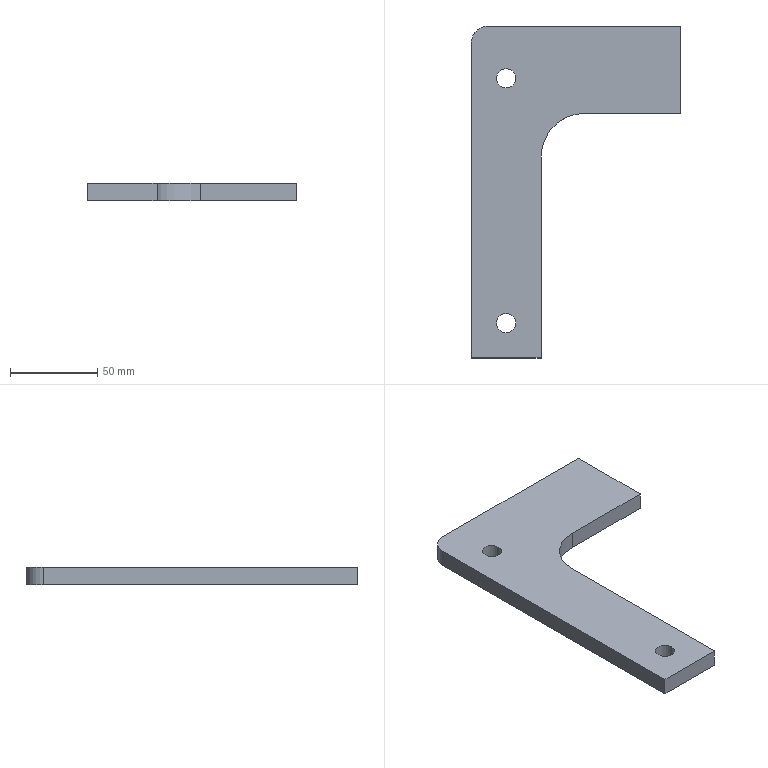Part | SolidWorks | features MBimport 1 | 1 solid | 14 faces | box 120 x 190 x 10 mm | volume 115226 mm3 | plane 8 | cylinder 6 | commonest cylinder face diameters 11 x4 20 x1 50 x1
STEP:
#1=CARTESIAN_POINT('',(-24.249,-90.402,10.));
#2=VERTEX_POINT('',#1);
#3=CARTESIAN_POINT('',(-24.249,-90.402,0.));
#4=VERTEX_POINT('',#3);
#5=CARTESIAN_POINT('',(-24.249,-90.402,10.));
#6=DIRECTION('',(0.,0.,-1.));
#7=VECTOR('',#6,1000.);
#8=LINE('',#5,#7);
#9=EDGE_CURVE('',#2,#4,#8,.T.);
#10=ORIENTED_EDGE('',*,*,#9,.F.);
#11=CARTESIAN_POINT('',(-35.249,-90.402,10.));
#12=VERTEX_POINT('',#11);
#13=CARTESIAN_POINT('',(-29.749,-90.402,10.));
#14=DIRECTION('',(0.,0.,1.));
#15=DIRECTION('',(1.,0.,0.));
#16=AXIS2_PLACEMENT_3D('',#13,#14,#15);
#17=CIRCLE('',#16,5.5);
#18=EDGE_CURVE('',#2,#12,#17,.T.);
#19=ORIENTED_EDGE('',*,*,#18,.T.);
#20=CARTESIAN_POINT('',(-35.249,-90.402,0.));
#21=VERTEX_POINT('',#20);
#22=CARTESIAN_POINT('',(-35.249,-90.402,10.));
#23=DIRECTION('',(0.,0.,-1.));
#24=VECTOR('',#23,1000.);
#25=LINE('',#22,#24);
#26=EDGE_CURVE('',#12,#21,#25,.T.);
#27=ORIENTED_EDGE('',*,*,#26,.T.);
#28=CARTESIAN_POINT('',(-29.749,-90.402,0.));
#29=DIRECTION('',(0.,0.,1.));
#30=DIRECTION('',(1.,0.,0.));
#31=AXIS2_PLACEMENT_3D('',#28,#29,#30);
#32=CIRCLE('',#31,5.5);
#33=EDGE_CURVE('',#4,#21,#32,.T.);
#34=ORIENTED_EDGE('',*,*,#33,.F.);
#35=EDGE_LOOP('',(#10,#19,#27,#34));
#36=FACE_OUTER_BOUND('',#35,.T.);
#37=CARTESIAN_POINT('',(-29.749,-90.402,10.));
#38=DIRECTION('',(0.,0.,-1.));
#39=DIRECTION('',(-1.,0.,0.));
#40=AXIS2_PLACEMENT_3D('',#37,#38,#39);
#41=CYLINDRICAL_SURFACE('',#40,5.5);
#42=ADVANCED_FACE('',(#36),#41,.F.);
#43=CARTESIAN_POINT('',(-24.249,49.598,10.));
#44=VERTEX_POINT('',#43);
#45=CARTESIAN_POINT('',(-24.249,49.598,0.));
#46=VERTEX_POINT('',#45);
#47=CARTESIAN_POINT('',(-24.249,49.598,10.));
#48=DIRECTION('',(0.,0.,-1.));
#49=VECTOR('',#48,1000.);
#50=LINE('',#47,#49);
#51=EDGE_CURVE('',#44,#46,#50,.T.);
#52=ORIENTED_EDGE('',*,*,#51,.F.);
#53=CARTESIAN_POINT('',(-35.249,49.598,10.));
#54=VERTEX_POINT('',#53);
#55=CARTESIAN_POINT('',(-29.749,49.598,10.));
#56=DIRECTION('',(0.,0.,1.));
#57=DIRECTION('',(1.,0.,0.));
#58=AXIS2_PLACEMENT_3D('',#55,#56,#57);
#59=CIRCLE('',#58,5.5);
#60=EDGE_CURVE('',#44,#54,#59,.T.);
#61=ORIENTED_EDGE('',*,*,#60,.T.);
#62=CARTESIAN_POINT('',(-35.249,49.598,0.));
#63=VERTEX_POINT('',#62);
#64=CARTESIAN_POINT('',(-35.249,49.598,10.));
#65=DIRECTION('',(0.,0.,-1.));
#66=VECTOR('',#65,1000.);
#67=LINE('',#64,#66);
#68=EDGE_CURVE('',#54,#63,#67,.T.);
#69=ORIENTED_EDGE('',*,*,#68,.T.);
#70=CARTESIAN_POINT('',(-29.749,49.598,0.));
#71=DIRECTION('',(0.,0.,1.));
#72=DIRECTION('',(1.,0.,0.));
#73=AXIS2_PLACEMENT_3D('',#70,#71,#72);
#74=CIRCLE('',#73,5.5);
#75=EDGE_CURVE('',#46,#63,#74,.T.);
#76=ORIENTED_EDGE('',*,*,#75,.F.);
#77=EDGE_LOOP('',(#52,#61,#69,#76));
#78=FACE_OUTER_BOUND('',#77,.T.);
#79=CARTESIAN_POINT('',(-29.749,49.598,10.));
#80=DIRECTION('',(0.,0.,-1.));
#81=DIRECTION('',(-1.,0.,0.));
#82=AXIS2_PLACEMENT_3D('',#79,#80,#81);
#83=CYLINDRICAL_SURFACE('',#82,5.5);
#84=ADVANCED_FACE('',(#78),#83,.F.);
#85=CARTESIAN_POINT('',(-49.749,69.598,0.));
#86=VERTEX_POINT('',#85);
#87=CARTESIAN_POINT('',(-49.749,-110.402,0.));
#88=VERTEX_POINT('',#87);
#89=CARTESIAN_POINT('',(-49.749,69.598,0.));
#90=DIRECTION('',(0.,-1.,0.));
#91=VECTOR('',#90,1000.);
#92=LINE('',#89,#91);
#93=EDGE_CURVE('',#86,#88,#92,.T.);
#94=ORIENTED_EDGE('',*,*,#93,.T.);
#95=CARTESIAN_POINT('',(-49.749,-110.402,10.));
#96=VERTEX_POINT('',#95);
#97=CARTESIAN_POINT('',(-49.749,-110.402,10.));
#98=DIRECTION('',(0.,0.,-1.));
#99=VECTOR('',#98,1000.);
#100=LINE('',#97,#99);
#101=EDGE_CURVE('',#96,#88,#100,.T.);
#102=ORIENTED_EDGE('',*,*,#101,.F.);
#103=CARTESIAN_POINT('',(-49.749,69.598,10.));
#104=VERTEX_POINT('',#103);
#105=CARTESIAN_POINT('',(-49.749,69.598,10.));
#106=DIRECTION('',(0.,-1.,0.));
#107=VECTOR('',#106,1000.);
#108=LINE('',#105,#107);
#109=EDGE_CURVE('',#104,#96,#108,.T.);
#110=ORIENTED_EDGE('',*,*,#109,.F.);
#111=CARTESIAN_POINT('',(-49.749,69.598,10.));
#112=DIRECTION('',(0.,0.,-1.));
#113=VECTOR('',#112,1000.);
#114=LINE('',#111,#113);
#115=EDGE_CURVE('',#104,#86,#114,.T.);
#116=ORIENTED_EDGE('',*,*,#115,.T.);
#117=EDGE_LOOP('',(#94,#102,#110,#116));
#118=FACE_OUTER_BOUND('',#117,.T.);
#119=CARTESIAN_POINT('',(-49.749,69.598,10.));
#120=DIRECTION('',(1.,0.,0.));
#121=DIRECTION('',(0.,1.,0.));
#122=AXIS2_PLACEMENT_3D('',#119,#120,#121);
#123=PLANE('',#122);
#124=ADVANCED_FACE('',(#118),#123,.F.);
#125=CARTESIAN_POINT('',(-39.749,79.598,0.));
#126=VERTEX_POINT('',#125);
#127=CARTESIAN_POINT('',(-39.749,69.598,0.));
#128=DIRECTION('',(0.,0.,1.));
#129=DIRECTION('',(-1.,0.,0.));
#130=AXIS2_PLACEMENT_3D('',#127,#128,#129);
#131=CIRCLE('',#130,10.);
#132=EDGE_CURVE('',#126,#86,#131,.T.);
#133=ORIENTED_EDGE('',*,*,#132,.T.);
#134=ORIENTED_EDGE('',*,*,#115,.F.);
#135=CARTESIAN_POINT('',(-39.749,79.598,10.));
#136=VERTEX_POINT('',#135);
#137=CARTESIAN_POINT('',(-39.749,69.598,10.));
#138=DIRECTION('',(0.,0.,1.));
#139=DIRECTION('',(-1.,0.,0.));
#140=AXIS2_PLACEMENT_3D('',#137,#138,#139);
#141=CIRCLE('',#140,10.);
#142=EDGE_CURVE('',#136,#104,#141,.T.);
#143=ORIENTED_EDGE('',*,*,#142,.F.);
#144=CARTESIAN_POINT('',(-39.749,79.598,10.));
#145=DIRECTION('',(0.,0.,-1.));
#146=VECTOR('',#145,1000.);
#147=LINE('',#144,#146);
#148=EDGE_CURVE('',#136,#126,#147,.T.);
#149=ORIENTED_EDGE('',*,*,#148,.T.);
#150=EDGE_LOOP('',(#133,#134,#143,#149));
#151=FACE_OUTER_BOUND('',#150,.T.);
#152=CARTESIAN_POINT('',(-39.749,69.598,10.));
#153=DIRECTION('',(0.,0.,-1.));
#154=DIRECTION('',(-1.,0.,0.));
#155=AXIS2_PLACEMENT_3D('',#152,#153,#154);
#156=CYLINDRICAL_SURFACE('',#155,10.);
#157=ADVANCED_FACE('',(#151),#156,.T.);
#158=CARTESIAN_POINT('',(70.251,79.598,0.));
#159=VERTEX_POINT('',#158);
#160=CARTESIAN_POINT('',(70.251,79.598,0.));
#161=DIRECTION('',(-1.,0.,0.));
#162=VECTOR('',#161,1000.);
#163=LINE('',#160,#162);
#164=EDGE_CURVE('',#159,#126,#163,.T.);
#165=ORIENTED_EDGE('',*,*,#164,.T.);
#166=ORIENTED_EDGE('',*,*,#148,.F.);
#167=CARTESIAN_POINT('',(70.251,79.598,10.));
#168=VERTEX_POINT('',#167);
#169=CARTESIAN_POINT('',(70.251,79.598,10.));
#170=DIRECTION('',(-1.,0.,0.));
#171=VECTOR('',#170,1000.);
#172=LINE('',#169,#171);
#173=EDGE_CURVE('',#168,#136,#172,.T.);
#174=ORIENTED_EDGE('',*,*,#173,.F.);
#175=CARTESIAN_POINT('',(70.251,79.598,10.));
#176=DIRECTION('',(0.,0.,-1.));
#177=VECTOR('',#176,1000.);
#178=LINE('',#175,#177);
#179=EDGE_CURVE('',#168,#159,#178,.T.);
#180=ORIENTED_EDGE('',*,*,#179,.T.);
#181=EDGE_LOOP('',(#165,#166,#174,#180));
#182=FACE_OUTER_BOUND('',#181,.T.);
#183=CARTESIAN_POINT('',(70.251,79.598,10.));
#184=DIRECTION('',(0.,-1.,0.));
#185=DIRECTION('',(0.,0.,-1.));
#186=AXIS2_PLACEMENT_3D('',#183,#184,#185);
#187=PLANE('',#186);
#188=ADVANCED_FACE('',(#182),#187,.F.);
#189=CARTESIAN_POINT('',(70.251,29.598,0.));
#190=VERTEX_POINT('',#189);
#191=CARTESIAN_POINT('',(70.251,29.598,0.));
#192=DIRECTION('',(0.,1.,0.));
#193=VECTOR('',#192,1000.);
#194=LINE('',#191,#193);
#195=EDGE_CURVE('',#190,#159,#194,.T.);
#196=ORIENTED_EDGE('',*,*,#195,.T.);
#197=ORIENTED_EDGE('',*,*,#179,.F.);
#198=CARTESIAN_POINT('',(70.251,29.598,10.));
#199=VERTEX_POINT('',#198);
#200=CARTESIAN_POINT('',(70.251,29.598,10.));
#201=DIRECTION('',(0.,1.,0.));
#202=VECTOR('',#201,1000.);
#203=LINE('',#200,#202);
#204=EDGE_CURVE('',#199,#168,#203,.T.);
#205=ORIENTED_EDGE('',*,*,#204,.F.);
#206=CARTESIAN_POINT('',(70.251,29.598,10.));
#207=DIRECTION('',(0.,0.,-1.));
#208=VECTOR('',#207,1000.);
#209=LINE('',#206,#208);
#210=EDGE_CURVE('',#199,#190,#209,.T.);
#211=ORIENTED_EDGE('',*,*,#210,.T.);
#212=EDGE_LOOP('',(#196,#197,#205,#211));
#213=FACE_OUTER_BOUND('',#212,.T.);
#214=CARTESIAN_POINT('',(70.251,29.598,10.));
#215=DIRECTION('',(-1.,0.,0.));
#216=DIRECTION('',(0.,0.,1.));
#217=AXIS2_PLACEMENT_3D('',#214,#215,#216);
#218=PLANE('',#217);
#219=ADVANCED_FACE('',(#213),#218,.F.);
#220=CARTESIAN_POINT('',(15.251,29.598,0.));
#221=VERTEX_POINT('',#220);
#222=CARTESIAN_POINT('',(15.251,29.598,0.));
#223=DIRECTION('',(1.,0.,0.));
#224=VECTOR('',#223,1000.);
#225=LINE('',#222,#224);
#226=EDGE_CURVE('',#221,#190,#225,.T.);
#227=ORIENTED_EDGE('',*,*,#226,.T.);
#228=ORIENTED_EDGE('',*,*,#210,.F.);
#229=CARTESIAN_POINT('',(15.251,29.598,10.));
#230=VERTEX_POINT('',#229);
#231=CARTESIAN_POINT('',(15.251,29.598,10.));
#232=DIRECTION('',(1.,0.,0.));
#233=VECTOR('',#232,1000.);
#234=LINE('',#231,#233);
#235=EDGE_CURVE('',#230,#199,#234,.T.);
#236=ORIENTED_EDGE('',*,*,#235,.F.);
#237=CARTESIAN_POINT('',(15.251,29.598,10.));
#238=DIRECTION('',(0.,0.,-1.));
#239=VECTOR('',#238,1000.);
#240=LINE('',#237,#239);
#241=EDGE_CURVE('',#230,#221,#240,.T.);
#242=ORIENTED_EDGE('',*,*,#241,.T.);
#243=EDGE_LOOP('',(#227,#228,#236,#242));
#244=FACE_OUTER_BOUND('',#243,.T.);
#245=CARTESIAN_POINT('',(15.251,29.598,10.));
#246=DIRECTION('',(0.,1.,0.));
#247=DIRECTION('',(1.,0.,0.));
#248=AXIS2_PLACEMENT_3D('',#245,#246,#247);
#249=PLANE('',#248);
#250=ADVANCED_FACE('',(#244),#249,.F.);
#251=CARTESIAN_POINT('',(-9.749,4.598,0.));
#252=VERTEX_POINT('',#251);
#253=CARTESIAN_POINT('',(15.251,4.598,0.));
#254=DIRECTION('',(0.,0.,-1.));
#255=DIRECTION('',(-1.,0.,0.));
#256=AXIS2_PLACEMENT_3D('',#253,#254,#255);
#257=CIRCLE('',#256,25.);
#258=EDGE_CURVE('',#252,#221,#257,.T.);
#259=ORIENTED_EDGE('',*,*,#258,.T.);
#260=ORIENTED_EDGE('',*,*,#241,.F.);
#261=CARTESIAN_POINT('',(-9.749,4.598,10.));
#262=VERTEX_POINT('',#261);
#263=CARTESIAN_POINT('',(15.251,4.598,10.));
#264=DIRECTION('',(0.,0.,-1.));
#265=DIRECTION('',(-1.,0.,0.));
#266=AXIS2_PLACEMENT_3D('',#263,#264,#265);
#267=CIRCLE('',#266,25.);
#268=EDGE_CURVE('',#262,#230,#267,.T.);
#269=ORIENTED_EDGE('',*,*,#268,.F.);
#270=CARTESIAN_POINT('',(-9.749,4.598,10.));
#271=DIRECTION('',(0.,0.,-1.));
#272=VECTOR('',#271,1000.);
#273=LINE('',#270,#272);
#274=EDGE_CURVE('',#262,#252,#273,.T.);
#275=ORIENTED_EDGE('',*,*,#274,.T.);
#276=EDGE_LOOP('',(#259,#260,#269,#275));
#277=FACE_OUTER_BOUND('',#276,.T.);
#278=CARTESIAN_POINT('',(15.251,4.598,10.));
#279=DIRECTION('',(0.,0.,-1.));
#280=DIRECTION('',(-1.,0.,0.));
#281=AXIS2_PLACEMENT_3D('',#278,#279,#280);
#282=CYLINDRICAL_SURFACE('',#281,25.);
#283=ADVANCED_FACE('',(#277),#282,.F.);
#284=CARTESIAN_POINT('',(-9.749,-110.402,0.));
#285=VERTEX_POINT('',#284);
#286=CARTESIAN_POINT('',(-9.749,-110.402,0.));
#287=DIRECTION('',(0.,1.,0.));
#288=VECTOR('',#287,1000.);
#289=LINE('',#286,#288);
#290=EDGE_CURVE('',#285,#252,#289,.T.);
#291=ORIENTED_EDGE('',*,*,#290,.T.);
#292=ORIENTED_EDGE('',*,*,#274,.F.);
#293=CARTESIAN_POINT('',(-9.749,-110.402,10.));
#294=VERTEX_POINT('',#293);
#295=CARTESIAN_POINT('',(-9.749,-110.402,10.));
#296=DIRECTION('',(0.,1.,0.));
#297=VECTOR('',#296,1000.);
#298=LINE('',#295,#297);
#299=EDGE_CURVE('',#294,#262,#298,.T.);
#300=ORIENTED_EDGE('',*,*,#299,.F.);
#301=CARTESIAN_POINT('',(-9.749,-110.402,10.));
#302=DIRECTION('',(0.,0.,-1.));
#303=VECTOR('',#302,1000.);
#304=LINE('',#301,#303);
#305=EDGE_CURVE('',#294,#285,#304,.T.);
#306=ORIENTED_EDGE('',*,*,#305,.T.);
#307=EDGE_LOOP('',(#291,#292,#300,#306));
#308=FACE_OUTER_BOUND('',#307,.T.);
#309=CARTESIAN_POINT('',(-9.749,-110.402,10.));
#310=DIRECTION('',(-1.,0.,0.));
#311=DIRECTION('',(0.,1.,0.));
#312=AXIS2_PLACEMENT_3D('',#309,#310,#311);
#313=PLANE('',#312);
#314=ADVANCED_FACE('',(#308),#313,.F.);
#315=CARTESIAN_POINT('',(-49.749,-110.402,0.));
#316=DIRECTION('',(1.,0.,0.));
#317=VECTOR('',#316,1000.);
#318=LINE('',#315,#317);
#319=EDGE_CURVE('',#88,#285,#318,.T.);
#320=ORIENTED_EDGE('',*,*,#319,.T.);
#321=ORIENTED_EDGE('',*,*,#305,.F.);
#322=CARTESIAN_POINT('',(-49.749,-110.402,10.));
#323=DIRECTION('',(1.,0.,0.));
#324=VECTOR('',#323,1000.);
#325=LINE('',#322,#324);
#326=EDGE_CURVE('',#96,#294,#325,.T.);
#327=ORIENTED_EDGE('',*,*,#326,.F.);
#328=ORIENTED_EDGE('',*,*,#101,.T.);
#329=EDGE_LOOP('',(#320,#321,#327,#328));
#330=FACE_OUTER_BOUND('',#329,.T.);
#331=CARTESIAN_POINT('',(-49.749,-110.402,10.));
#332=DIRECTION('',(0.,1.,0.));
#333=DIRECTION('',(1.,0.,0.));
#334=AXIS2_PLACEMENT_3D('',#331,#332,#333);
#335=PLANE('',#334);
#336=ADVANCED_FACE('',(#330),#335,.F.);
#337=CARTESIAN_POINT('',(-29.749,-90.402,0.));
#338=DIRECTION('',(0.,0.,1.));
#339=DIRECTION('',(1.,0.,0.));
#340=AXIS2_PLACEMENT_3D('',#337,#338,#339);
#341=CIRCLE('',#340,5.5);
#342=EDGE_CURVE('',#21,#4,#341,.T.);
#343=ORIENTED_EDGE('',*,*,#342,.T.);
#344=ORIENTED_EDGE('',*,*,#33,.T.);
#345=EDGE_LOOP('',(#343,#344));
#346=FACE_BOUND('',#345,.T.);
#347=CARTESIAN_POINT('',(-29.749,49.598,0.));
#348=DIRECTION('',(0.,0.,1.));
#349=DIRECTION('',(1.,0.,0.));
#350=AXIS2_PLACEMENT_3D('',#347,#348,#349);
#351=CIRCLE('',#350,5.5);
#352=EDGE_CURVE('',#63,#46,#351,.T.);
#353=ORIENTED_EDGE('',*,*,#352,.T.);
#354=ORIENTED_EDGE('',*,*,#75,.T.);
#355=EDGE_LOOP('',(#353,#354));
#356=FACE_BOUND('',#355,.T.);
#357=ORIENTED_EDGE('',*,*,#319,.F.);
#358=ORIENTED_EDGE('',*,*,#93,.F.);
#359=ORIENTED_EDGE('',*,*,#132,.F.);
#360=ORIENTED_EDGE('',*,*,#164,.F.);
#361=ORIENTED_EDGE('',*,*,#195,.F.);
#362=ORIENTED_EDGE('',*,*,#226,.F.);
#363=ORIENTED_EDGE('',*,*,#258,.F.);
#364=ORIENTED_EDGE('',*,*,#290,.F.);
#365=EDGE_LOOP('',(#357,#358,#359,#360,#361,#362,#363,#364));
#366=FACE_OUTER_BOUND('',#365,.T.);
#367=CARTESIAN_POINT('',(15.251,4.598,0.));
#368=DIRECTION('',(0.,0.,-1.));
#369=DIRECTION('',(0.,-1.,0.));
#370=AXIS2_PLACEMENT_3D('',#367,#368,#369);
#371=PLANE('',#370);
#372=ADVANCED_FACE('',(#346,#356,#366),#371,.T.);
#373=CARTESIAN_POINT('',(-29.749,-90.402,10.));
#374=DIRECTION('',(0.,0.,1.));
#375=DIRECTION('',(1.,0.,0.));
#376=AXIS2_PLACEMENT_3D('',#373,#374,#375);
#377=CIRCLE('',#376,5.5);
#378=EDGE_CURVE('',#12,#2,#377,.T.);
#379=ORIENTED_EDGE('',*,*,#378,.F.);
#380=ORIENTED_EDGE('',*,*,#18,.F.);
#381=EDGE_LOOP('',(#379,#380));
#382=FACE_BOUND('',#381,.T.);
#383=CARTESIAN_POINT('',(-29.749,49.598,10.));
#384=DIRECTION('',(0.,0.,1.));
#385=DIRECTION('',(1.,0.,0.));
#386=AXIS2_PLACEMENT_3D('',#383,#384,#385);
#387=CIRCLE('',#386,5.5);
#388=EDGE_CURVE('',#54,#44,#387,.T.);
#389=ORIENTED_EDGE('',*,*,#388,.F.);
#390=ORIENTED_EDGE('',*,*,#60,.F.);
#391=EDGE_LOOP('',(#389,#390));
#392=FACE_BOUND('',#391,.T.);
#393=ORIENTED_EDGE('',*,*,#326,.T.);
#394=ORIENTED_EDGE('',*,*,#299,.T.);
#395=ORIENTED_EDGE('',*,*,#268,.T.);
#396=ORIENTED_EDGE('',*,*,#235,.T.);
#397=ORIENTED_EDGE('',*,*,#204,.T.);
#398=ORIENTED_EDGE('',*,*,#173,.T.);
#399=ORIENTED_EDGE('',*,*,#142,.T.);
#400=ORIENTED_EDGE('',*,*,#109,.T.);
#401=EDGE_LOOP('',(#393,#394,#395,#396,#397,#398,#399,#400));
#402=FACE_OUTER_BOUND('',#401,.T.);
#403=CARTESIAN_POINT('',(15.251,4.598,10.));
#404=DIRECTION('',(0.,0.,-1.));
#405=DIRECTION('',(0.,-1.,0.));
#406=AXIS2_PLACEMENT_3D('',#403,#404,#405);
#407=PLANE('',#406);
#408=ADVANCED_FACE('',(#382,#392,#402),#407,.F.);
#409=ORIENTED_EDGE('',*,*,#388,.T.);
#410=ORIENTED_EDGE('',*,*,#51,.T.);
#411=ORIENTED_EDGE('',*,*,#352,.F.);
#412=ORIENTED_EDGE('',*,*,#68,.F.);
#413=EDGE_LOOP('',(#409,#410,#411,#412));
#414=FACE_OUTER_BOUND('',#413,.T.);
#415=CARTESIAN_POINT('',(-29.749,49.598,10.));
#416=DIRECTION('',(0.,0.,-1.));
#417=DIRECTION('',(-1.,0.,0.));
#418=AXIS2_PLACEMENT_3D('',#415,#416,#417);
#419=CYLINDRICAL_SURFACE('',#418,5.5);
#420=ADVANCED_FACE('',(#414),#419,.F.);
#421=ORIENTED_EDGE('',*,*,#378,.T.);
#422=ORIENTED_EDGE('',*,*,#9,.T.);
#423=ORIENTED_EDGE('',*,*,#342,.F.);
#424=ORIENTED_EDGE('',*,*,#26,.F.);
#425=EDGE_LOOP('',(#421,#422,#423,#424));
#426=FACE_OUTER_BOUND('',#425,.T.);
#427=CARTESIAN_POINT('',(-29.749,-90.402,10.));
#428=DIRECTION('',(0.,0.,-1.));
#429=DIRECTION('',(-1.,0.,0.));
#430=AXIS2_PLACEMENT_3D('',#427,#428,#429);
#431=CYLINDRICAL_SURFACE('',#430,5.5);
#432=ADVANCED_FACE('',(#426),#431,.F.);
#433=CLOSED_SHELL('',(#42,#84,#124,#157,#188,#219,#250,#283,#314,#336,#372,#408,#420,#432));
#434=MANIFOLD_SOLID_BREP('',#433);
#435=CARTESIAN_POINT('',(0.,0.,0.));
#436=DIRECTION('',(0.,0.,1.));
#437=DIRECTION('',(1.,0.,0.));
#438=AXIS2_PLACEMENT_3D('',#435,#436,#437);
#439=(LENGTH_UNIT()NAMED_UNIT(*)SI_UNIT(.MILLI.,.METRE.));
#440=UNCERTAINTY_MEASURE_WITH_UNIT(LENGTH_MEASURE(0.00001),#439,'','');
#441=(NAMED_UNIT(*)PLANE_ANGLE_UNIT()SI_UNIT($,.RADIAN.));
#442=(NAMED_UNIT(*)SI_UNIT($,.STERADIAN.)SOLID_ANGLE_UNIT());
#443=(GEOMETRIC_REPRESENTATION_CONTEXT(3)GLOBAL_UNCERTAINTY_ASSIGNED_CONTEXT((#440))GLOBAL_UNIT_ASSIGNED_CONTEXT((#439,#441,#442))REPRESENTATION_CONTEXT('',''));
#444=ADVANCED_BREP_SHAPE_REPRESENTATION('',(#434,#438),#443);